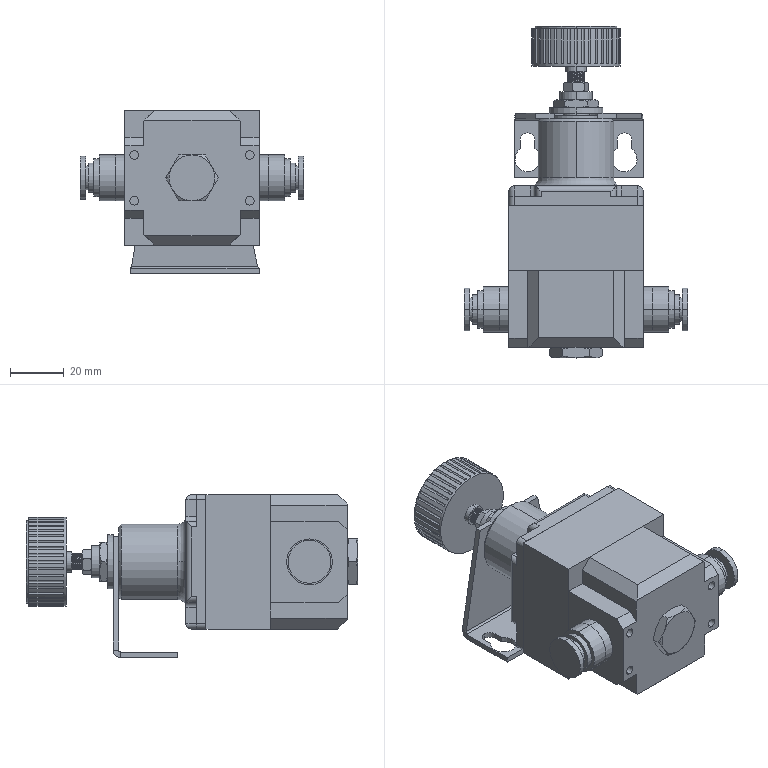Part | SolidWorks | 5 solids | 378 faces | box 83 x 123.4 x 60.54 mm | volume 179227 mm3 | cylinder 161 | plane 159 | cone 52 | spline 4 | torus 2 | commonest cylinder face diameters 0.887 x59 4 x20 6 x18 3.3 x8 5.5 x4 7.9 x4